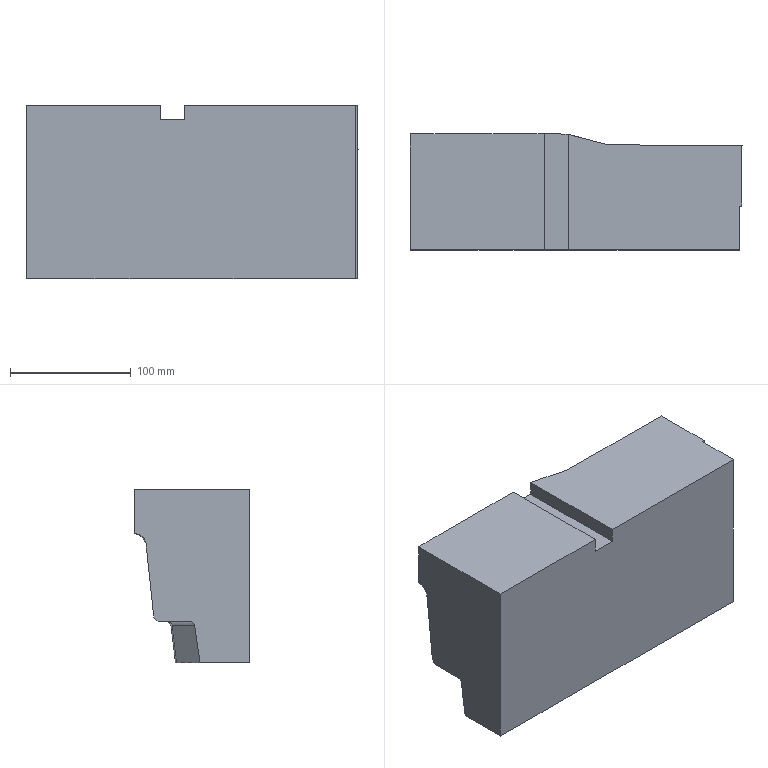Part | NX | features solid 2 | 1 solid | 47 faces | volume 3018327 mm3 | spline 34 | plane 13